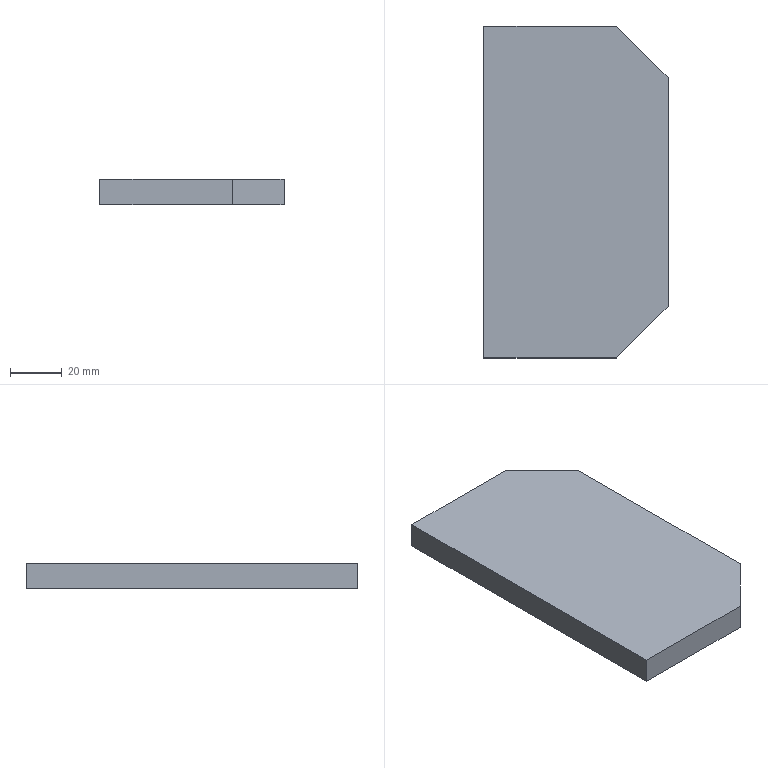Part | STEP file | 06 Rib plate | 1 solid | 8 faces | box 71 x 128 x 10 mm | volume 86880 mm3 | plane 8
STEP:
#1=CARTESIAN_POINT('',(0.,0.,0.));
#2=DIRECTION('',(0.,0.,1.));
#3=DIRECTION('',(1.,0.,0.));
#4=AXIS2_PLACEMENT_3D('',#1,#2,#3);
#5=CARTESIAN_POINT('',(0.,0.,0.));
#6=VERTEX_POINT('',#5);
#7=CARTESIAN_POINT('',(0.,-128.,0.));
#8=VERTEX_POINT('',#7);
#9=CARTESIAN_POINT('',(0.,0.,0.));
#10=DIRECTION('',(0.,-1.,0.));
#11=VECTOR('',#10,1.);
#12=LINE('',#9,#11);
#13=CARTESIAN_POINT('',(0.,0.,10.));
#14=DIRECTION('',(1.,0.,0.));
#15=DIRECTION('',(0.,1.,0.));
#16=AXIS2_PLACEMENT_3D('',#13,#14,#15);
#17=PLANE('',#16);
#18=CARTESIAN_POINT('',(0.,-10.));
#19=DIRECTION('',(-1.,0.));
#20=VECTOR('',#19,1.);
#21=LINE('',#18,#20);
#22=(GEOMETRIC_REPRESENTATION_CONTEXT(2)PARAMETRIC_REPRESENTATION_CONTEXT()REPRESENTATION_CONTEXT('',''));
#23=DEFINITIONAL_REPRESENTATION('',(#21),#22);
#24=PCURVE('',#17,#23);
#25=CARTESIAN_POINT('',(0.,0.,0.));
#26=DIRECTION('',(0.,0.,1.));
#27=DIRECTION('',(1.,0.,0.));
#28=AXIS2_PLACEMENT_3D('',#25,#26,#27);
#29=PLANE('',#28);
#30=CARTESIAN_POINT('',(0.,0.));
#31=DIRECTION('',(0.,-1.));
#32=VECTOR('',#31,1.);
#33=LINE('',#30,#32);
#34=(GEOMETRIC_REPRESENTATION_CONTEXT(2)PARAMETRIC_REPRESENTATION_CONTEXT()REPRESENTATION_CONTEXT('',''));
#35=DEFINITIONAL_REPRESENTATION('',(#33),#34);
#36=PCURVE('',#29,#35);
#37=SURFACE_CURVE('',#12,(#24,#36),.PCURVE_S1.);
#38=EDGE_CURVE('',#6,#8,#37,.T.);
#39=ORIENTED_EDGE('',*,*,#38,.T.);
#40=CARTESIAN_POINT('',(0.,-128.,10.));
#41=VERTEX_POINT('',#40);
#42=CARTESIAN_POINT('',(0.,-128.,10.));
#43=DIRECTION('',(0.,0.,-1.));
#44=VECTOR('',#43,1.);
#45=LINE('',#42,#44);
#46=CARTESIAN_POINT('',(-128.,0.));
#47=DIRECTION('',(0.,-1.));
#48=VECTOR('',#47,1.);
#49=LINE('',#46,#48);
#50=(GEOMETRIC_REPRESENTATION_CONTEXT(2)PARAMETRIC_REPRESENTATION_CONTEXT()REPRESENTATION_CONTEXT('',''));
#51=DEFINITIONAL_REPRESENTATION('',(#49),#50);
#52=PCURVE('',#17,#51);
#53=CARTESIAN_POINT('',(0.,-128.,10.));
#54=DIRECTION('',(0.,1.,0.));
#55=DIRECTION('',(0.,0.,1.));
#56=AXIS2_PLACEMENT_3D('',#53,#54,#55);
#57=PLANE('',#56);
#58=CARTESIAN_POINT('',(0.,0.));
#59=DIRECTION('',(-1.,0.));
#60=VECTOR('',#59,1.);
#61=LINE('',#58,#60);
#62=(GEOMETRIC_REPRESENTATION_CONTEXT(2)PARAMETRIC_REPRESENTATION_CONTEXT()REPRESENTATION_CONTEXT('',''));
#63=DEFINITIONAL_REPRESENTATION('',(#61),#62);
#64=PCURVE('',#57,#63);
#65=SURFACE_CURVE('',#45,(#52,#64),.PCURVE_S1.);
#66=EDGE_CURVE('',#41,#8,#65,.T.);
#67=ORIENTED_EDGE('',*,*,#66,.F.);
#68=CARTESIAN_POINT('',(0.,0.,10.));
#69=VERTEX_POINT('',#68);
#70=CARTESIAN_POINT('',(0.,0.,10.));
#71=DIRECTION('',(0.,-1.,0.));
#72=VECTOR('',#71,1.);
#73=LINE('',#70,#72);
#74=CARTESIAN_POINT('',(0.,0.));
#75=DIRECTION('',(-1.,0.));
#76=VECTOR('',#75,1.);
#77=LINE('',#74,#76);
#78=(GEOMETRIC_REPRESENTATION_CONTEXT(2)PARAMETRIC_REPRESENTATION_CONTEXT()REPRESENTATION_CONTEXT('',''));
#79=DEFINITIONAL_REPRESENTATION('',(#77),#78);
#80=PCURVE('',#17,#79);
#81=CARTESIAN_POINT('',(0.,0.,10.));
#82=DIRECTION('',(0.,0.,1.));
#83=DIRECTION('',(1.,0.,0.));
#84=AXIS2_PLACEMENT_3D('',#81,#82,#83);
#85=PLANE('',#84);
#86=CARTESIAN_POINT('',(0.,0.));
#87=DIRECTION('',(0.,-1.));
#88=VECTOR('',#87,1.);
#89=LINE('',#86,#88);
#90=(GEOMETRIC_REPRESENTATION_CONTEXT(2)PARAMETRIC_REPRESENTATION_CONTEXT()REPRESENTATION_CONTEXT('',''));
#91=DEFINITIONAL_REPRESENTATION('',(#89),#90);
#92=PCURVE('',#85,#91);
#93=SURFACE_CURVE('',#73,(#80,#92),.PCURVE_S1.);
#94=EDGE_CURVE('',#69,#41,#93,.T.);
#95=ORIENTED_EDGE('',*,*,#94,.F.);
#96=CARTESIAN_POINT('',(0.,0.,10.));
#97=DIRECTION('',(0.,0.,-1.));
#98=VECTOR('',#97,1.);
#99=LINE('',#96,#98);
#100=CARTESIAN_POINT('',(0.,0.));
#101=DIRECTION('',(0.,-1.));
#102=VECTOR('',#101,1.);
#103=LINE('',#100,#102);
#104=(GEOMETRIC_REPRESENTATION_CONTEXT(2)PARAMETRIC_REPRESENTATION_CONTEXT()REPRESENTATION_CONTEXT('',''));
#105=DEFINITIONAL_REPRESENTATION('',(#103),#104);
#106=PCURVE('',#17,#105);
#107=CARTESIAN_POINT('',(0.,0.,10.));
#108=DIRECTION('',(0.,-1.,0.));
#109=DIRECTION('',(0.,0.,-1.));
#110=AXIS2_PLACEMENT_3D('',#107,#108,#109);
#111=PLANE('',#110);
#112=CARTESIAN_POINT('',(0.,0.));
#113=DIRECTION('',(1.,0.));
#114=VECTOR('',#113,1.);
#115=LINE('',#112,#114);
#116=(GEOMETRIC_REPRESENTATION_CONTEXT(2)PARAMETRIC_REPRESENTATION_CONTEXT()REPRESENTATION_CONTEXT('',''));
#117=DEFINITIONAL_REPRESENTATION('',(#115),#116);
#118=PCURVE('',#111,#117);
#119=SURFACE_CURVE('',#99,(#106,#118),.PCURVE_S1.);
#120=EDGE_CURVE('',#69,#6,#119,.T.);
#121=ORIENTED_EDGE('',*,*,#120,.T.);
#122=EDGE_LOOP('',(#39,#67,#95,#121));
#123=FACE_BOUND('',#122,.T.);
#124=ADVANCED_FACE('',(#123),#17,.F.);
#125=CARTESIAN_POINT('',(51.,-128.,0.));
#126=VERTEX_POINT('',#125);
#127=CARTESIAN_POINT('',(0.,-128.,0.));
#128=DIRECTION('',(1.,0.,0.));
#129=VECTOR('',#128,1.);
#130=LINE('',#127,#129);
#131=CARTESIAN_POINT('',(-10.,0.));
#132=DIRECTION('',(0.,1.));
#133=VECTOR('',#132,1.);
#134=LINE('',#131,#133);
#135=(GEOMETRIC_REPRESENTATION_CONTEXT(2)PARAMETRIC_REPRESENTATION_CONTEXT()REPRESENTATION_CONTEXT('',''));
#136=DEFINITIONAL_REPRESENTATION('',(#134),#135);
#137=PCURVE('',#57,#136);
#138=CARTESIAN_POINT('',(0.,-128.));
#139=DIRECTION('',(1.,0.));
#140=VECTOR('',#139,1.);
#141=LINE('',#138,#140);
#142=(GEOMETRIC_REPRESENTATION_CONTEXT(2)PARAMETRIC_REPRESENTATION_CONTEXT()REPRESENTATION_CONTEXT('',''));
#143=DEFINITIONAL_REPRESENTATION('',(#141),#142);
#144=PCURVE('',#29,#143);
#145=SURFACE_CURVE('',#130,(#137,#144),.PCURVE_S1.);
#146=EDGE_CURVE('',#8,#126,#145,.T.);
#147=ORIENTED_EDGE('',*,*,#146,.T.);
#148=CARTESIAN_POINT('',(51.,-128.,10.));
#149=VERTEX_POINT('',#148);
#150=CARTESIAN_POINT('',(51.,-128.,10.));
#151=DIRECTION('',(0.,0.,-1.));
#152=VECTOR('',#151,1.);
#153=LINE('',#150,#152);
#154=CARTESIAN_POINT('',(0.,51.));
#155=DIRECTION('',(-1.,0.));
#156=VECTOR('',#155,1.);
#157=LINE('',#154,#156);
#158=(GEOMETRIC_REPRESENTATION_CONTEXT(2)PARAMETRIC_REPRESENTATION_CONTEXT()REPRESENTATION_CONTEXT('',''));
#159=DEFINITIONAL_REPRESENTATION('',(#157),#158);
#160=PCURVE('',#57,#159);
#161=CARTESIAN_POINT('',(71.,-108.,10.));
#162=DIRECTION('',(-0.7071,0.7071,0.));
#163=DIRECTION('',(-0.7071,-0.7071,0.));
#164=AXIS2_PLACEMENT_3D('',#161,#162,#163);
#165=PLANE('',#164);
#166=CARTESIAN_POINT('',(28.284,0.));
#167=DIRECTION('',(0.,-1.));
#168=VECTOR('',#167,1.);
#169=LINE('',#166,#168);
#170=(GEOMETRIC_REPRESENTATION_CONTEXT(2)PARAMETRIC_REPRESENTATION_CONTEXT()REPRESENTATION_CONTEXT('',''));
#171=DEFINITIONAL_REPRESENTATION('',(#169),#170);
#172=PCURVE('',#165,#171);
#173=SURFACE_CURVE('',#153,(#160,#172),.PCURVE_S1.);
#174=EDGE_CURVE('',#149,#126,#173,.T.);
#175=ORIENTED_EDGE('',*,*,#174,.F.);
#176=CARTESIAN_POINT('',(0.,-128.,10.));
#177=DIRECTION('',(1.,0.,0.));
#178=VECTOR('',#177,1.);
#179=LINE('',#176,#178);
#180=CARTESIAN_POINT('',(0.,0.));
#181=DIRECTION('',(0.,1.));
#182=VECTOR('',#181,1.);
#183=LINE('',#180,#182);
#184=(GEOMETRIC_REPRESENTATION_CONTEXT(2)PARAMETRIC_REPRESENTATION_CONTEXT()REPRESENTATION_CONTEXT('',''));
#185=DEFINITIONAL_REPRESENTATION('',(#183),#184);
#186=PCURVE('',#57,#185);
#187=CARTESIAN_POINT('',(0.,-128.));
#188=DIRECTION('',(1.,0.));
#189=VECTOR('',#188,1.);
#190=LINE('',#187,#189);
#191=(GEOMETRIC_REPRESENTATION_CONTEXT(2)PARAMETRIC_REPRESENTATION_CONTEXT()REPRESENTATION_CONTEXT('',''));
#192=DEFINITIONAL_REPRESENTATION('',(#190),#191);
#193=PCURVE('',#85,#192);
#194=SURFACE_CURVE('',#179,(#186,#193),.PCURVE_S1.);
#195=EDGE_CURVE('',#41,#149,#194,.T.);
#196=ORIENTED_EDGE('',*,*,#195,.F.);
#197=ORIENTED_EDGE('',*,*,#66,.T.);
#198=EDGE_LOOP('',(#147,#175,#196,#197));
#199=FACE_BOUND('',#198,.T.);
#200=ADVANCED_FACE('',(#199),#57,.F.);
#201=CARTESIAN_POINT('',(71.,-108.,0.));
#202=VERTEX_POINT('',#201);
#203=CARTESIAN_POINT('',(71.,-108.,0.));
#204=DIRECTION('',(0.7071,0.7071,0.));
#205=VECTOR('',#204,1.);
#206=LINE('',#203,#205);
#207=CARTESIAN_POINT('',(0.,-10.));
#208=DIRECTION('',(-1.,0.));
#209=VECTOR('',#208,1.);
#210=LINE('',#207,#209);
#211=(GEOMETRIC_REPRESENTATION_CONTEXT(2)PARAMETRIC_REPRESENTATION_CONTEXT()REPRESENTATION_CONTEXT('',''));
#212=DEFINITIONAL_REPRESENTATION('',(#210),#211);
#213=PCURVE('',#165,#212);
#214=CARTESIAN_POINT('',(71.,-108.));
#215=DIRECTION('',(0.7071,0.7071));
#216=VECTOR('',#215,1.);
#217=LINE('',#214,#216);
#218=(GEOMETRIC_REPRESENTATION_CONTEXT(2)PARAMETRIC_REPRESENTATION_CONTEXT()REPRESENTATION_CONTEXT('',''));
#219=DEFINITIONAL_REPRESENTATION('',(#217),#218);
#220=PCURVE('',#29,#219);
#221=SURFACE_CURVE('',#206,(#213,#220),.PCURVE_S1.);
#222=EDGE_CURVE('',#126,#202,#221,.T.);
#223=ORIENTED_EDGE('',*,*,#222,.T.);
#224=CARTESIAN_POINT('',(71.,-108.,10.));
#225=VERTEX_POINT('',#224);
#226=CARTESIAN_POINT('',(71.,-108.,10.));
#227=DIRECTION('',(0.,0.,-1.));
#228=VECTOR('',#227,1.);
#229=LINE('',#226,#228);
#230=CARTESIAN_POINT('',(0.,0.));
#231=DIRECTION('',(0.,-1.));
#232=VECTOR('',#231,1.);
#233=LINE('',#230,#232);
#234=(GEOMETRIC_REPRESENTATION_CONTEXT(2)PARAMETRIC_REPRESENTATION_CONTEXT()REPRESENTATION_CONTEXT('',''));
#235=DEFINITIONAL_REPRESENTATION('',(#233),#234);
#236=PCURVE('',#165,#235);
#237=CARTESIAN_POINT('',(71.,-20.,10.));
#238=DIRECTION('',(-1.,0.,0.));
#239=DIRECTION('',(0.,-1.,0.));
#240=AXIS2_PLACEMENT_3D('',#237,#238,#239);
#241=PLANE('',#240);
#242=CARTESIAN_POINT('',(88.,0.));
#243=DIRECTION('',(0.,-1.));
#244=VECTOR('',#243,1.);
#245=LINE('',#242,#244);
#246=(GEOMETRIC_REPRESENTATION_CONTEXT(2)PARAMETRIC_REPRESENTATION_CONTEXT()REPRESENTATION_CONTEXT('',''));
#247=DEFINITIONAL_REPRESENTATION('',(#245),#246);
#248=PCURVE('',#241,#247);
#249=SURFACE_CURVE('',#229,(#236,#248),.PCURVE_S1.);
#250=EDGE_CURVE('',#225,#202,#249,.T.);
#251=ORIENTED_EDGE('',*,*,#250,.F.);
#252=CARTESIAN_POINT('',(71.,-108.,10.));
#253=DIRECTION('',(0.7071,0.7071,0.));
#254=VECTOR('',#253,1.);
#255=LINE('',#252,#254);
#256=CARTESIAN_POINT('',(0.,0.));
#257=DIRECTION('',(-1.,0.));
#258=VECTOR('',#257,1.);
#259=LINE('',#256,#258);
#260=(GEOMETRIC_REPRESENTATION_CONTEXT(2)PARAMETRIC_REPRESENTATION_CONTEXT()REPRESENTATION_CONTEXT('',''));
#261=DEFINITIONAL_REPRESENTATION('',(#259),#260);
#262=PCURVE('',#165,#261);
#263=CARTESIAN_POINT('',(71.,-108.));
#264=DIRECTION('',(0.7071,0.7071));
#265=VECTOR('',#264,1.);
#266=LINE('',#263,#265);
#267=(GEOMETRIC_REPRESENTATION_CONTEXT(2)PARAMETRIC_REPRESENTATION_CONTEXT()REPRESENTATION_CONTEXT('',''));
#268=DEFINITIONAL_REPRESENTATION('',(#266),#267);
#269=PCURVE('',#85,#268);
#270=SURFACE_CURVE('',#255,(#262,#269),.PCURVE_S1.);
#271=EDGE_CURVE('',#149,#225,#270,.T.);
#272=ORIENTED_EDGE('',*,*,#271,.F.);
#273=ORIENTED_EDGE('',*,*,#174,.T.);
#274=EDGE_LOOP('',(#223,#251,#272,#273));
#275=FACE_BOUND('',#274,.T.);
#276=ADVANCED_FACE('',(#275),#165,.F.);
#277=CARTESIAN_POINT('',(71.,-20.,0.));
#278=VERTEX_POINT('',#277);
#279=CARTESIAN_POINT('',(71.,-20.,0.));
#280=DIRECTION('',(0.,1.,0.));
#281=VECTOR('',#280,1.);
#282=LINE('',#279,#281);
#283=CARTESIAN_POINT('',(0.,-10.));
#284=DIRECTION('',(-1.,0.));
#285=VECTOR('',#284,1.);
#286=LINE('',#283,#285);
#287=(GEOMETRIC_REPRESENTATION_CONTEXT(2)PARAMETRIC_REPRESENTATION_CONTEXT()REPRESENTATION_CONTEXT('',''));
#288=DEFINITIONAL_REPRESENTATION('',(#286),#287);
#289=PCURVE('',#241,#288);
#290=CARTESIAN_POINT('',(71.,-20.));
#291=DIRECTION('',(0.,1.));
#292=VECTOR('',#291,1.);
#293=LINE('',#290,#292);
#294=(GEOMETRIC_REPRESENTATION_CONTEXT(2)PARAMETRIC_REPRESENTATION_CONTEXT()REPRESENTATION_CONTEXT('',''));
#295=DEFINITIONAL_REPRESENTATION('',(#293),#294);
#296=PCURVE('',#29,#295);
#297=SURFACE_CURVE('',#282,(#289,#296),.PCURVE_S1.);
#298=EDGE_CURVE('',#202,#278,#297,.T.);
#299=ORIENTED_EDGE('',*,*,#298,.T.);
#300=CARTESIAN_POINT('',(71.,-20.,10.));
#301=VERTEX_POINT('',#300);
#302=CARTESIAN_POINT('',(71.,-20.,10.));
#303=DIRECTION('',(0.,0.,-1.));
#304=VECTOR('',#303,1.);
#305=LINE('',#302,#304);
#306=CARTESIAN_POINT('',(0.,0.));
#307=DIRECTION('',(0.,-1.));
#308=VECTOR('',#307,1.);
#309=LINE('',#306,#308);
#310=(GEOMETRIC_REPRESENTATION_CONTEXT(2)PARAMETRIC_REPRESENTATION_CONTEXT()REPRESENTATION_CONTEXT('',''));
#311=DEFINITIONAL_REPRESENTATION('',(#309),#310);
#312=PCURVE('',#241,#311);
#313=CARTESIAN_POINT('',(51.,0.,10.));
#314=DIRECTION('',(-0.7071,-0.7071,0.));
#315=DIRECTION('',(0.7071,-0.7071,0.));
#316=AXIS2_PLACEMENT_3D('',#313,#314,#315);
#317=PLANE('',#316);
#318=CARTESIAN_POINT('',(28.284,0.));
#319=DIRECTION('',(0.,-1.));
#320=VECTOR('',#319,1.);
#321=LINE('',#318,#320);
#322=(GEOMETRIC_REPRESENTATION_CONTEXT(2)PARAMETRIC_REPRESENTATION_CONTEXT()REPRESENTATION_CONTEXT('',''));
#323=DEFINITIONAL_REPRESENTATION('',(#321),#322);
#324=PCURVE('',#317,#323);
#325=SURFACE_CURVE('',#305,(#312,#324),.PCURVE_S1.);
#326=EDGE_CURVE('',#301,#278,#325,.T.);
#327=ORIENTED_EDGE('',*,*,#326,.F.);
#328=CARTESIAN_POINT('',(71.,-20.,10.));
#329=DIRECTION('',(0.,1.,0.));
#330=VECTOR('',#329,1.);
#331=LINE('',#328,#330);
#332=CARTESIAN_POINT('',(0.,0.));
#333=DIRECTION('',(-1.,0.));
#334=VECTOR('',#333,1.);
#335=LINE('',#332,#334);
#336=(GEOMETRIC_REPRESENTATION_CONTEXT(2)PARAMETRIC_REPRESENTATION_CONTEXT()REPRESENTATION_CONTEXT('',''));
#337=DEFINITIONAL_REPRESENTATION('',(#335),#336);
#338=PCURVE('',#241,#337);
#339=CARTESIAN_POINT('',(71.,-20.));
#340=DIRECTION('',(0.,1.));
#341=VECTOR('',#340,1.);
#342=LINE('',#339,#341);
#343=(GEOMETRIC_REPRESENTATION_CONTEXT(2)PARAMETRIC_REPRESENTATION_CONTEXT()REPRESENTATION_CONTEXT('',''));
#344=DEFINITIONAL_REPRESENTATION('',(#342),#343);
#345=PCURVE('',#85,#344);
#346=SURFACE_CURVE('',#331,(#338,#345),.PCURVE_S1.);
#347=EDGE_CURVE('',#225,#301,#346,.T.);
#348=ORIENTED_EDGE('',*,*,#347,.F.);
#349=ORIENTED_EDGE('',*,*,#250,.T.);
#350=EDGE_LOOP('',(#299,#327,#348,#349));
#351=FACE_BOUND('',#350,.T.);
#352=ADVANCED_FACE('',(#351),#241,.F.);
#353=CARTESIAN_POINT('',(51.,0.,0.));
#354=VERTEX_POINT('',#353);
#355=CARTESIAN_POINT('',(51.,0.,0.));
#356=DIRECTION('',(-0.7071,0.7071,0.));
#357=VECTOR('',#356,1.);
#358=LINE('',#355,#357);
#359=CARTESIAN_POINT('',(0.,-10.));
#360=DIRECTION('',(-1.,0.));
#361=VECTOR('',#360,1.);
#362=LINE('',#359,#361);
#363=(GEOMETRIC_REPRESENTATION_CONTEXT(2)PARAMETRIC_REPRESENTATION_CONTEXT()REPRESENTATION_CONTEXT('',''));
#364=DEFINITIONAL_REPRESENTATION('',(#362),#363);
#365=PCURVE('',#317,#364);
#366=CARTESIAN_POINT('',(51.,0.));
#367=DIRECTION('',(-0.7071,0.7071));
#368=VECTOR('',#367,1.);
#369=LINE('',#366,#368);
#370=(GEOMETRIC_REPRESENTATION_CONTEXT(2)PARAMETRIC_REPRESENTATION_CONTEXT()REPRESENTATION_CONTEXT('',''));
#371=DEFINITIONAL_REPRESENTATION('',(#369),#370);
#372=PCURVE('',#29,#371);
#373=SURFACE_CURVE('',#358,(#365,#372),.PCURVE_S1.);
#374=EDGE_CURVE('',#278,#354,#373,.T.);
#375=ORIENTED_EDGE('',*,*,#374,.T.);
#376=CARTESIAN_POINT('',(51.,0.,10.));
#377=VERTEX_POINT('',#376);
#378=CARTESIAN_POINT('',(51.,0.,10.));
#379=DIRECTION('',(0.,0.,-1.));
#380=VECTOR('',#379,1.);
#381=LINE('',#378,#380);
#382=CARTESIAN_POINT('',(0.,0.));
#383=DIRECTION('',(0.,-1.));
#384=VECTOR('',#383,1.);
#385=LINE('',#382,#384);
#386=(GEOMETRIC_REPRESENTATION_CONTEXT(2)PARAMETRIC_REPRESENTATION_CONTEXT()REPRESENTATION_CONTEXT('',''));
#387=DEFINITIONAL_REPRESENTATION('',(#385),#386);
#388=PCURVE('',#317,#387);
#389=CARTESIAN_POINT('',(0.,51.));
#390=DIRECTION('',(1.,0.));
#391=VECTOR('',#390,1.);
#392=LINE('',#389,#391);
#393=(GEOMETRIC_REPRESENTATION_CONTEXT(2)PARAMETRIC_REPRESENTATION_CONTEXT()REPRESENTATION_CONTEXT('',''));
#394=DEFINITIONAL_REPRESENTATION('',(#392),#393);
#395=PCURVE('',#111,#394);
#396=SURFACE_CURVE('',#381,(#388,#395),.PCURVE_S1.);
#397=EDGE_CURVE('',#377,#354,#396,.T.);
#398=ORIENTED_EDGE('',*,*,#397,.F.);
#399=CARTESIAN_POINT('',(51.,0.,10.));
#400=DIRECTION('',(-0.7071,0.7071,0.));
#401=VECTOR('',#400,1.);
#402=LINE('',#399,#401);
#403=CARTESIAN_POINT('',(0.,0.));
#404=DIRECTION('',(-1.,0.));
#405=VECTOR('',#404,1.);
#406=LINE('',#403,#405);
#407=(GEOMETRIC_REPRESENTATION_CONTEXT(2)PARAMETRIC_REPRESENTATION_CONTEXT()REPRESENTATION_CONTEXT('',''));
#408=DEFINITIONAL_REPRESENTATION('',(#406),#407);
#409=PCURVE('',#317,#408);
#410=CARTESIAN_POINT('',(51.,0.));
#411=DIRECTION('',(-0.7071,0.7071));
#412=VECTOR('',#411,1.);
#413=LINE('',#410,#412);
#414=(GEOMETRIC_REPRESENTATION_CONTEXT(2)PARAMETRIC_REPRESENTATION_CONTEXT()REPRESENTATION_CONTEXT('',''));
#415=DEFINITIONAL_REPRESENTATION('',(#413),#414);
#416=PCURVE('',#85,#415);
#417=SURFACE_CURVE('',#402,(#409,#416),.PCURVE_S1.);
#418=EDGE_CURVE('',#301,#377,#417,.T.);
#419=ORIENTED_EDGE('',*,*,#418,.F.);
#420=ORIENTED_EDGE('',*,*,#326,.T.);
#421=EDGE_LOOP('',(#375,#398,#419,#420));
#422=FACE_BOUND('',#421,.T.);
#423=ADVANCED_FACE('',(#422),#317,.F.);
#424=CARTESIAN_POINT('',(0.,0.,0.));
#425=DIRECTION('',(-1.,0.,0.));
#426=VECTOR('',#425,1.);
#427=LINE('',#424,#426);
#428=CARTESIAN_POINT('',(10.,0.));
#429=DIRECTION('',(0.,-1.));
#430=VECTOR('',#429,1.);
#431=LINE('',#428,#430);
#432=(GEOMETRIC_REPRESENTATION_CONTEXT(2)PARAMETRIC_REPRESENTATION_CONTEXT()REPRESENTATION_CONTEXT('',''));
#433=DEFINITIONAL_REPRESENTATION('',(#431),#432);
#434=PCURVE('',#111,#433);
#435=CARTESIAN_POINT('',(0.,0.));
#436=DIRECTION('',(-1.,0.));
#437=VECTOR('',#436,1.);
#438=LINE('',#435,#437);
#439=(GEOMETRIC_REPRESENTATION_CONTEXT(2)PARAMETRIC_REPRESENTATION_CONTEXT()REPRESENTATION_CONTEXT('',''));
#440=DEFINITIONAL_REPRESENTATION('',(#438),#439);
#441=PCURVE('',#29,#440);
#442=SURFACE_CURVE('',#427,(#434,#441),.PCURVE_S1.);
#443=EDGE_CURVE('',#354,#6,#442,.T.);
#444=ORIENTED_EDGE('',*,*,#443,.T.);
#445=ORIENTED_EDGE('',*,*,#120,.F.);
#446=CARTESIAN_POINT('',(0.,0.,10.));
#447=DIRECTION('',(-1.,0.,0.));
#448=VECTOR('',#447,1.);
#449=LINE('',#446,#448);
#450=CARTESIAN_POINT('',(0.,0.));
#451=DIRECTION('',(0.,-1.));
#452=VECTOR('',#451,1.);
#453=LINE('',#450,#452);
#454=(GEOMETRIC_REPRESENTATION_CONTEXT(2)PARAMETRIC_REPRESENTATION_CONTEXT()REPRESENTATION_CONTEXT('',''));
#455=DEFINITIONAL_REPRESENTATION('',(#453),#454);
#456=PCURVE('',#111,#455);
#457=CARTESIAN_POINT('',(0.,0.));
#458=DIRECTION('',(-1.,0.));
#459=VECTOR('',#458,1.);
#460=LINE('',#457,#459);
#461=(GEOMETRIC_REPRESENTATION_CONTEXT(2)PARAMETRIC_REPRESENTATION_CONTEXT()REPRESENTATION_CONTEXT('',''));
#462=DEFINITIONAL_REPRESENTATION('',(#460),#461);
#463=PCURVE('',#85,#462);
#464=SURFACE_CURVE('',#449,(#456,#463),.PCURVE_S1.);
#465=EDGE_CURVE('',#377,#69,#464,.T.);
#466=ORIENTED_EDGE('',*,*,#465,.F.);
#467=ORIENTED_EDGE('',*,*,#397,.T.);
#468=EDGE_LOOP('',(#444,#445,#466,#467));
#469=FACE_BOUND('',#468,.T.);
#470=ADVANCED_FACE('',(#469),#111,.F.);
#471=ORIENTED_EDGE('',*,*,#94,.T.);
#472=ORIENTED_EDGE('',*,*,#195,.T.);
#473=ORIENTED_EDGE('',*,*,#271,.T.);
#474=ORIENTED_EDGE('',*,*,#347,.T.);
#475=ORIENTED_EDGE('',*,*,#418,.T.);
#476=ORIENTED_EDGE('',*,*,#465,.T.);
#477=EDGE_LOOP('',(#471,#472,#473,#474,#475,#476));
#478=FACE_BOUND('',#477,.T.);
#479=ADVANCED_FACE('',(#478),#85,.T.);
#480=ORIENTED_EDGE('',*,*,#38,.F.);
#481=ORIENTED_EDGE('',*,*,#443,.F.);
#482=ORIENTED_EDGE('',*,*,#374,.F.);
#483=ORIENTED_EDGE('',*,*,#298,.F.);
#484=ORIENTED_EDGE('',*,*,#222,.F.);
#485=ORIENTED_EDGE('',*,*,#146,.F.);
#486=EDGE_LOOP('',(#480,#481,#482,#483,#484,#485));
#487=FACE_BOUND('',#486,.T.);
#488=ADVANCED_FACE('',(#487),#29,.F.);
#489=CLOSED_SHELL('',(#124,#200,#276,#352,#423,#470,#479,#488));
#490=MANIFOLD_SOLID_BREP('',#489);
#491=(LENGTH_UNIT()NAMED_UNIT(*)SI_UNIT(.MILLI.,.METRE.));
#492=UNCERTAINTY_MEASURE_WITH_UNIT(LENGTH_MEASURE(0.0000001),#491,'','');
#493=(NAMED_UNIT(*)PLANE_ANGLE_UNIT()SI_UNIT($,.RADIAN.));
#494=(NAMED_UNIT(*)SI_UNIT($,.STERADIAN.)SOLID_ANGLE_UNIT());
#495=(GEOMETRIC_REPRESENTATION_CONTEXT(3)GLOBAL_UNCERTAINTY_ASSIGNED_CONTEXT((#492))GLOBAL_UNIT_ASSIGNED_CONTEXT((#491,#493,#494))REPRESENTATION_CONTEXT('',''));
#496=ADVANCED_BREP_SHAPE_REPRESENTATION('',(#4,#490),#495);